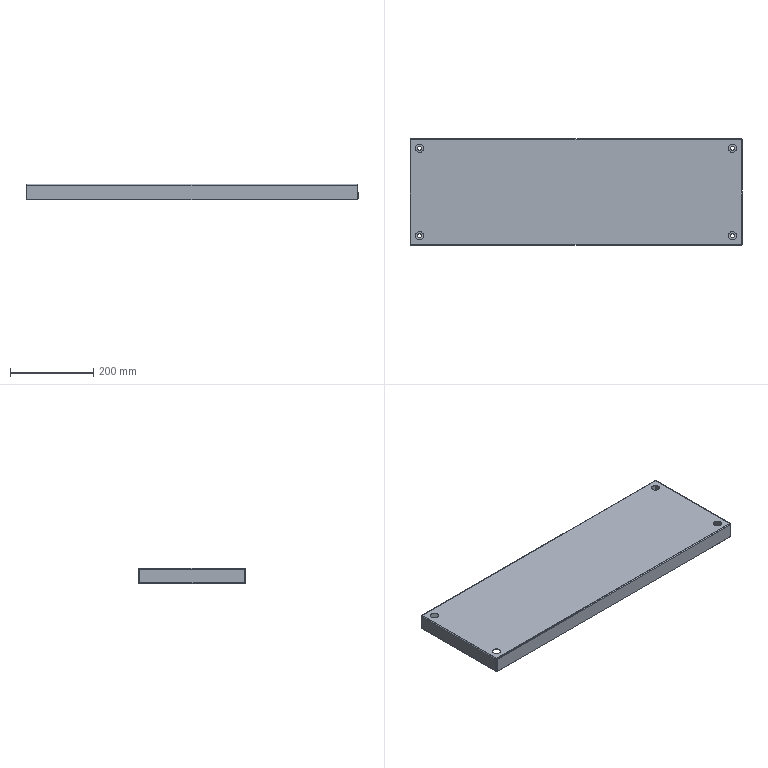Part | SolidWorks | features BaseBody 1 | 1 solid | 62 faces | box 796 x 256 x 37.5 mm | volume 442521 mm3 | cylinder 28 | plane 26 | spline 8 | commonest cylinder face diameters 10 x8 20 x8 1.473 x6 4.473 x6